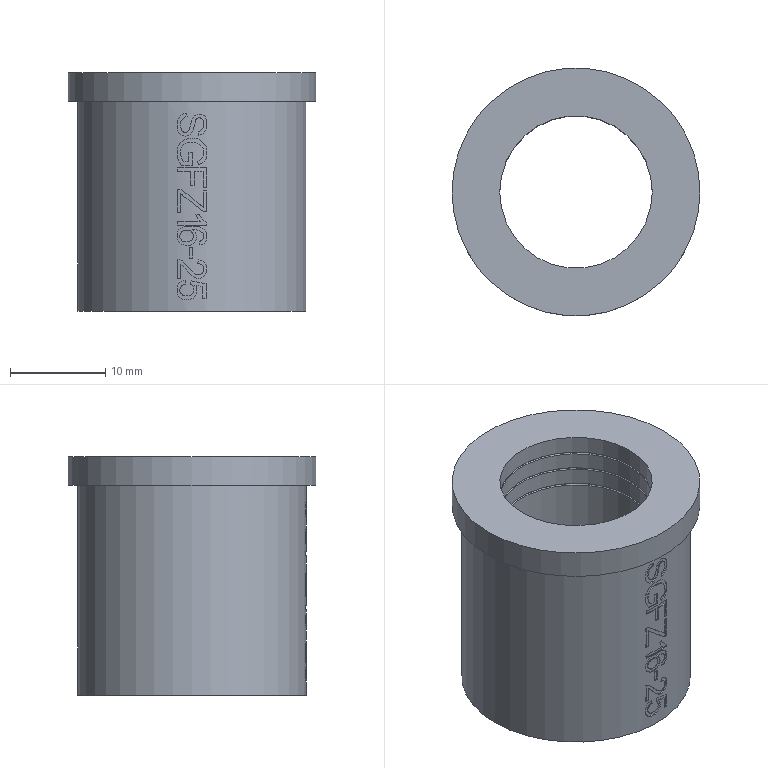Part | NX | features SGFZ16-25_1 2 | 1 solid | 137 faces | box 26 x 26 x 25 mm | volume 6514 mm3 | plane 79 | cylinder 55 | torus 3 | commonest cylinder face diameters 23.8 x9 16 x4 24 x2 0.853 x1 0.883 x1 1.056 x1